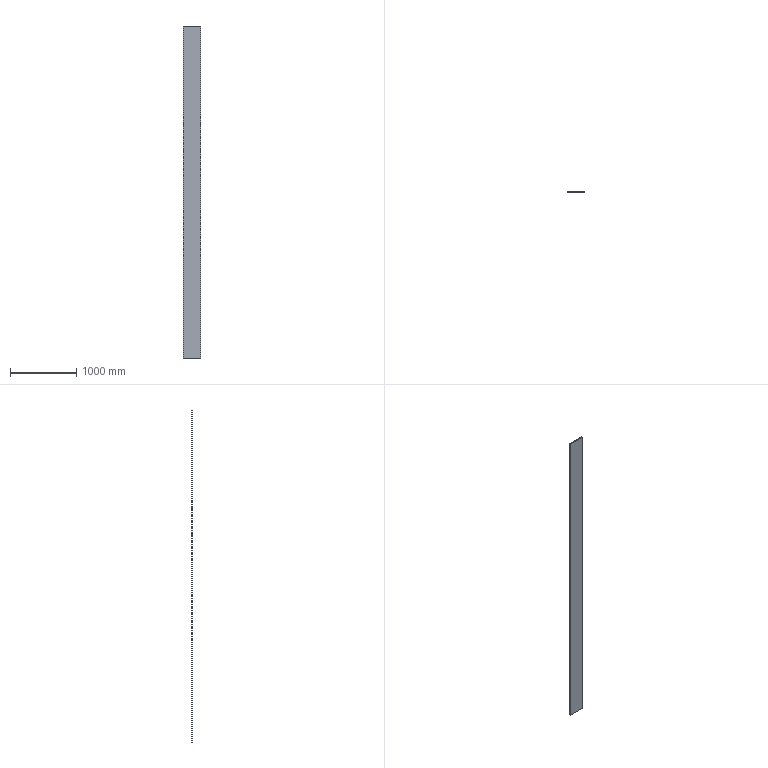Part | SolidWorks | features Extrusion 1 | 1 solid | 6 faces | box 260 x 10 x 5000 mm | volume 13000000 mm3 | plane 6
STEP:
#1=CARTESIAN_POINT('',(0.,10.,0.));
#2=VERTEX_POINT('',#1);
#3=CARTESIAN_POINT('',(0.,0.,0.));
#4=VERTEX_POINT('',#3);
#5=CARTESIAN_POINT('',(0.,0.,0.));
#6=DIRECTION('',(0.,-1.,0.));
#7=VECTOR('',#6,1000.);
#8=LINE('',#5,#7);
#9=EDGE_CURVE('',#2,#4,#8,.T.);
#10=ORIENTED_EDGE('',*,*,#9,.T.);
#11=CARTESIAN_POINT('',(0.,0.,5000.));
#12=VERTEX_POINT('',#11);
#13=CARTESIAN_POINT('',(0.,0.,5000.));
#14=DIRECTION('',(0.,0.,-1.));
#15=VECTOR('',#14,1000.);
#16=LINE('',#13,#15);
#17=EDGE_CURVE('',#12,#4,#16,.T.);
#18=ORIENTED_EDGE('',*,*,#17,.F.);
#19=CARTESIAN_POINT('',(0.,10.,5000.));
#20=VERTEX_POINT('',#19);
#21=CARTESIAN_POINT('',(0.,0.,5000.));
#22=DIRECTION('',(0.,-1.,0.));
#23=VECTOR('',#22,1000.);
#24=LINE('',#21,#23);
#25=EDGE_CURVE('',#20,#12,#24,.T.);
#26=ORIENTED_EDGE('',*,*,#25,.F.);
#27=CARTESIAN_POINT('',(0.,10.,5000.));
#28=DIRECTION('',(0.,0.,-1.));
#29=VECTOR('',#28,1000.);
#30=LINE('',#27,#29);
#31=EDGE_CURVE('',#20,#2,#30,.T.);
#32=ORIENTED_EDGE('',*,*,#31,.T.);
#33=EDGE_LOOP('',(#10,#18,#26,#32));
#34=FACE_OUTER_BOUND('',#33,.T.);
#35=CARTESIAN_POINT('',(0.,0.,5000.));
#36=DIRECTION('',(1.,0.,0.));
#37=DIRECTION('',(0.,0.,-1.));
#38=AXIS2_PLACEMENT_3D('',#35,#36,#37);
#39=PLANE('',#38);
#40=ADVANCED_FACE('',(#34),#39,.F.);
#41=CARTESIAN_POINT('',(260.,0.,0.));
#42=VERTEX_POINT('',#41);
#43=CARTESIAN_POINT('',(0.,0.,0.));
#44=DIRECTION('',(1.,0.,0.));
#45=VECTOR('',#44,1000.);
#46=LINE('',#43,#45);
#47=EDGE_CURVE('',#4,#42,#46,.T.);
#48=ORIENTED_EDGE('',*,*,#47,.T.);
#49=CARTESIAN_POINT('',(260.,0.,5000.));
#50=VERTEX_POINT('',#49);
#51=CARTESIAN_POINT('',(260.,0.,5000.));
#52=DIRECTION('',(0.,0.,-1.));
#53=VECTOR('',#52,1000.);
#54=LINE('',#51,#53);
#55=EDGE_CURVE('',#50,#42,#54,.T.);
#56=ORIENTED_EDGE('',*,*,#55,.F.);
#57=CARTESIAN_POINT('',(0.,0.,5000.));
#58=DIRECTION('',(1.,0.,0.));
#59=VECTOR('',#58,1000.);
#60=LINE('',#57,#59);
#61=EDGE_CURVE('',#12,#50,#60,.T.);
#62=ORIENTED_EDGE('',*,*,#61,.F.);
#63=ORIENTED_EDGE('',*,*,#17,.T.);
#64=EDGE_LOOP('',(#48,#56,#62,#63));
#65=FACE_OUTER_BOUND('',#64,.T.);
#66=CARTESIAN_POINT('',(0.,0.,5000.));
#67=DIRECTION('',(0.,1.,0.));
#68=DIRECTION('',(0.,0.,1.));
#69=AXIS2_PLACEMENT_3D('',#66,#67,#68);
#70=PLANE('',#69);
#71=ADVANCED_FACE('',(#65),#70,.F.);
#72=CARTESIAN_POINT('',(260.,10.,0.));
#73=VERTEX_POINT('',#72);
#74=CARTESIAN_POINT('',(260.,0.,0.));
#75=DIRECTION('',(0.,1.,0.));
#76=VECTOR('',#75,1000.);
#77=LINE('',#74,#76);
#78=EDGE_CURVE('',#42,#73,#77,.T.);
#79=ORIENTED_EDGE('',*,*,#78,.T.);
#80=CARTESIAN_POINT('',(260.,10.,5000.));
#81=VERTEX_POINT('',#80);
#82=CARTESIAN_POINT('',(260.,10.,5000.));
#83=DIRECTION('',(0.,0.,-1.));
#84=VECTOR('',#83,1000.);
#85=LINE('',#82,#84);
#86=EDGE_CURVE('',#81,#73,#85,.T.);
#87=ORIENTED_EDGE('',*,*,#86,.F.);
#88=CARTESIAN_POINT('',(260.,0.,5000.));
#89=DIRECTION('',(0.,1.,0.));
#90=VECTOR('',#89,1000.);
#91=LINE('',#88,#90);
#92=EDGE_CURVE('',#50,#81,#91,.T.);
#93=ORIENTED_EDGE('',*,*,#92,.F.);
#94=ORIENTED_EDGE('',*,*,#55,.T.);
#95=EDGE_LOOP('',(#79,#87,#93,#94));
#96=FACE_OUTER_BOUND('',#95,.T.);
#97=CARTESIAN_POINT('',(260.,0.,5000.));
#98=DIRECTION('',(-1.,0.,0.));
#99=DIRECTION('',(0.,0.,1.));
#100=AXIS2_PLACEMENT_3D('',#97,#98,#99);
#101=PLANE('',#100);
#102=ADVANCED_FACE('',(#96),#101,.F.);
#103=CARTESIAN_POINT('',(0.,10.,0.));
#104=DIRECTION('',(-1.,0.,0.));
#105=VECTOR('',#104,1000.);
#106=LINE('',#103,#105);
#107=EDGE_CURVE('',#73,#2,#106,.T.);
#108=ORIENTED_EDGE('',*,*,#107,.T.);
#109=ORIENTED_EDGE('',*,*,#31,.F.);
#110=CARTESIAN_POINT('',(0.,10.,5000.));
#111=DIRECTION('',(-1.,0.,0.));
#112=VECTOR('',#111,1000.);
#113=LINE('',#110,#112);
#114=EDGE_CURVE('',#81,#20,#113,.T.);
#115=ORIENTED_EDGE('',*,*,#114,.F.);
#116=ORIENTED_EDGE('',*,*,#86,.T.);
#117=EDGE_LOOP('',(#108,#109,#115,#116));
#118=FACE_OUTER_BOUND('',#117,.T.);
#119=CARTESIAN_POINT('',(0.,10.,5000.));
#120=DIRECTION('',(0.,-1.,0.));
#121=DIRECTION('',(0.,0.,-1.));
#122=AXIS2_PLACEMENT_3D('',#119,#120,#121);
#123=PLANE('',#122);
#124=ADVANCED_FACE('',(#118),#123,.F.);
#125=ORIENTED_EDGE('',*,*,#25,.T.);
#126=ORIENTED_EDGE('',*,*,#61,.T.);
#127=ORIENTED_EDGE('',*,*,#92,.T.);
#128=ORIENTED_EDGE('',*,*,#114,.T.);
#129=EDGE_LOOP('',(#125,#126,#127,#128));
#130=FACE_OUTER_BOUND('',#129,.T.);
#131=CARTESIAN_POINT('',(0.,0.,5000.));
#132=DIRECTION('',(0.,0.,-1.));
#133=DIRECTION('',(-1.,0.,0.));
#134=AXIS2_PLACEMENT_3D('',#131,#132,#133);
#135=PLANE('',#134);
#136=ADVANCED_FACE('',(#130),#135,.F.);
#137=ORIENTED_EDGE('',*,*,#9,.F.);
#138=ORIENTED_EDGE('',*,*,#107,.F.);
#139=ORIENTED_EDGE('',*,*,#78,.F.);
#140=ORIENTED_EDGE('',*,*,#47,.F.);
#141=EDGE_LOOP('',(#137,#138,#139,#140));
#142=FACE_OUTER_BOUND('',#141,.T.);
#143=CARTESIAN_POINT('',(0.,0.,0.));
#144=DIRECTION('',(0.,0.,-1.));
#145=DIRECTION('',(-1.,0.,0.));
#146=AXIS2_PLACEMENT_3D('',#143,#144,#145);
#147=PLANE('',#146);
#148=ADVANCED_FACE('',(#142),#147,.T.);
#149=CLOSED_SHELL('',(#40,#71,#102,#124,#136,#148));
#150=MANIFOLD_SOLID_BREP('',#149);
#151=CARTESIAN_POINT('',(0.,0.,0.));
#152=DIRECTION('',(0.,0.,1.));
#153=DIRECTION('',(1.,0.,0.));
#154=AXIS2_PLACEMENT_3D('',#151,#152,#153);
#155=(LENGTH_UNIT()NAMED_UNIT(*)SI_UNIT(.MILLI.,.METRE.));
#156=UNCERTAINTY_MEASURE_WITH_UNIT(LENGTH_MEASURE(0.00001),#155,'','');
#157=(NAMED_UNIT(*)PLANE_ANGLE_UNIT()SI_UNIT($,.RADIAN.));
#158=(NAMED_UNIT(*)SI_UNIT($,.STERADIAN.)SOLID_ANGLE_UNIT());
#159=(GEOMETRIC_REPRESENTATION_CONTEXT(3)GLOBAL_UNCERTAINTY_ASSIGNED_CONTEXT((#156))GLOBAL_UNIT_ASSIGNED_CONTEXT((#155,#157,#158))REPRESENTATION_CONTEXT('',''));
#160=ADVANCED_BREP_SHAPE_REPRESENTATION('',(#150,#154),#159);